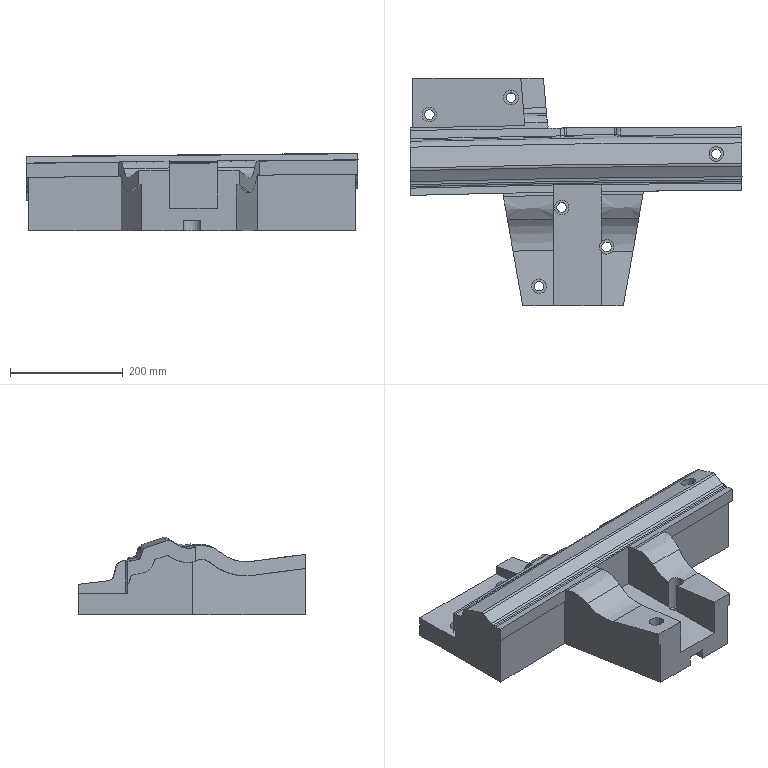Part | NX | features solid 2 | 1 solid | 133 faces | box 590.037 x 405 x 137.653 mm | volume 11662476 mm3 | spline 82 | plane 33 | cylinder 18 | commonest cylinder face diameters 17 x6 26 x6 32 x6